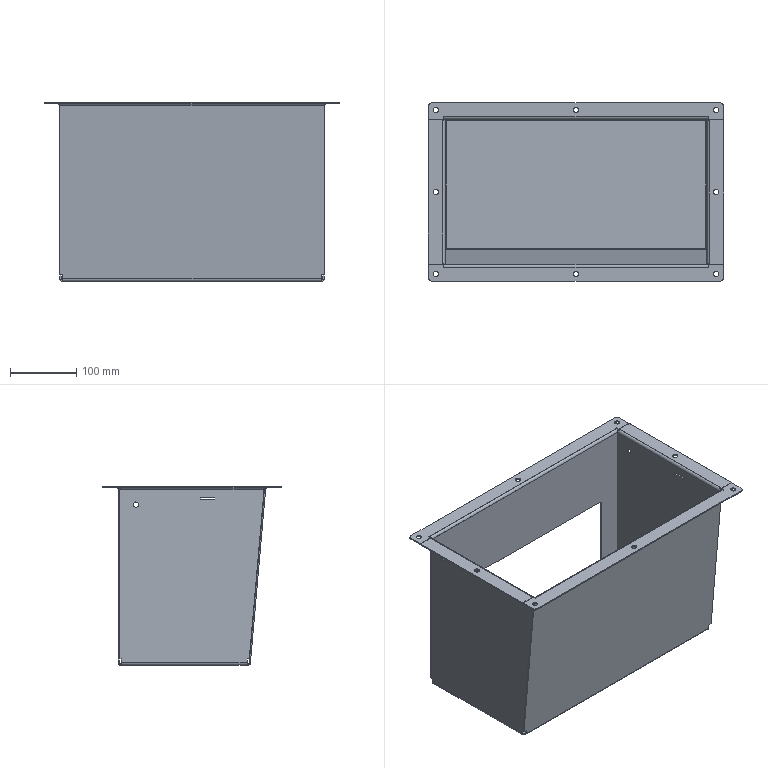Part | STEP file | SYL_0392D6J1SYL0380DJ100-698449 | 1 solid | 166 faces | box 446 x 269.609 x 269.8 mm | volume 707479 mm3 | plane 120 | cylinder 44 | spline 2 | commonest cylinder face diameters 8 x24 10 x8 4 x4 4.4 x4 7.6 x4